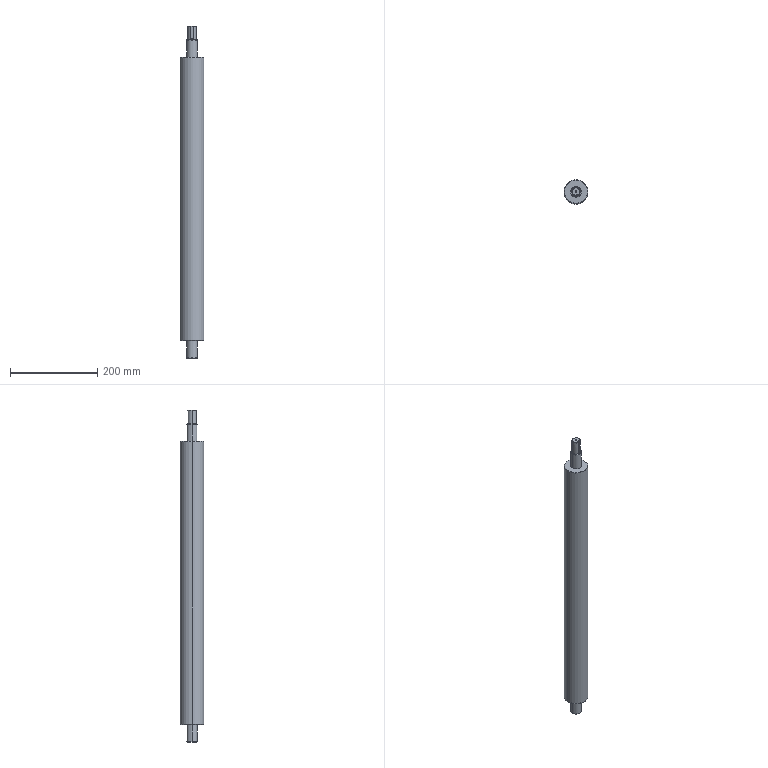Part | SolidWorks | features ICE 3, Chamfer 2, Extrusion 1, HoleWzd 1, MirrorPattern 1 | 1 solid | 32 faces | box 55 x 55 x 762 mm | volume 1592560 mm3 | cone 13 | cylinder 11 | plane 8 | commonest cylinder face diameters 25 x4 4.2 x2 20 x2 55 x2 6 x1
STEP:
#1=CARTESIAN_POINT('',(-2.1,0.,384.6));
#2=VERTEX_POINT('',#1);
#3=CARTESIAN_POINT('',(2.1,0.,384.6));
#4=VERTEX_POINT('',#3);
#5=CARTESIAN_POINT('',(0.,0.,384.6));
#6=DIRECTION('',(0.,0.,1.));
#7=DIRECTION('',(1.,0.,0.));
#8=AXIS2_PLACEMENT_3D('',#5,#6,#7);
#9=CIRCLE('',#8,2.1);
#10=EDGE_CURVE('',#2,#4,#9,.T.);
#11=ORIENTED_EDGE('',*,*,#10,.F.);
#12=CARTESIAN_POINT('',(-2.1,0.,397.));
#13=VERTEX_POINT('',#12);
#14=CARTESIAN_POINT('',(-2.1,0.,397.));
#15=DIRECTION('',(0.,0.,1.));
#16=VECTOR('',#15,1000.);
#17=LINE('',#14,#16);
#18=EDGE_CURVE('',#2,#13,#17,.T.);
#19=ORIENTED_EDGE('',*,*,#18,.T.);
#20=CARTESIAN_POINT('',(2.1,0.,397.));
#21=VERTEX_POINT('',#20);
#22=CARTESIAN_POINT('',(0.,0.,397.));
#23=DIRECTION('',(0.,0.,1.));
#24=DIRECTION('',(1.,0.,0.));
#25=AXIS2_PLACEMENT_3D('',#22,#23,#24);
#26=CIRCLE('',#25,2.1);
#27=EDGE_CURVE('',#13,#21,#26,.T.);
#28=ORIENTED_EDGE('',*,*,#27,.T.);
#29=CARTESIAN_POINT('',(2.1,0.,397.));
#30=DIRECTION('',(0.,0.,1.));
#31=VECTOR('',#30,1000.);
#32=LINE('',#29,#31);
#33=EDGE_CURVE('',#4,#21,#32,.T.);
#34=ORIENTED_EDGE('',*,*,#33,.F.);
#35=EDGE_LOOP('',(#11,#19,#28,#34));
#36=FACE_OUTER_BOUND('',#35,.T.);
#37=CARTESIAN_POINT('',(0.,0.,397.));
#38=DIRECTION('',(0.,0.,1.));
#39=DIRECTION('',(1.,0.,0.));
#40=AXIS2_PLACEMENT_3D('',#37,#38,#39);
#41=CYLINDRICAL_SURFACE('',#40,2.1);
#42=ADVANCED_FACE('',(#36),#41,.F.);
#43=CARTESIAN_POINT('',(0.,0.,383.338));
#44=VERTEX_POINT('',#43);
#45=CARTESIAN_POINT('',(2.1,0.,384.6));
#46=DIRECTION('',(0.8572,0.,0.515));
#47=VECTOR('',#46,1000.);
#48=LINE('',#45,#47);
#49=EDGE_CURVE('',#44,#4,#48,.T.);
#50=ORIENTED_EDGE('',*,*,#49,.F.);
#51=CARTESIAN_POINT('',(-2.1,0.,384.6));
#52=DIRECTION('',(-0.8572,0.,0.515));
#53=VECTOR('',#52,1000.);
#54=LINE('',#51,#53);
#55=EDGE_CURVE('',#44,#2,#54,.T.);
#56=ORIENTED_EDGE('',*,*,#55,.T.);
#57=ORIENTED_EDGE('',*,*,#10,.T.);
#58=EDGE_LOOP('',(#50,#56,#57));
#59=FACE_OUTER_BOUND('',#58,.T.);
#60=CARTESIAN_POINT('',(0.,0.,384.6));
#61=DIRECTION('',(0.,0.,1.));
#62=DIRECTION('',(1.,0.,0.));
#63=AXIS2_PLACEMENT_3D('',#60,#61,#62);
#64=CONICAL_SURFACE('',#63,2.1,1.03);
#65=ADVANCED_FACE('',(#59),#64,.F.);
#66=CARTESIAN_POINT('',(9.,0.,397.));
#67=VERTEX_POINT('',#66);
#68=CARTESIAN_POINT('',(-9.,0.,397.));
#69=VERTEX_POINT('',#68);
#70=CARTESIAN_POINT('',(0.,0.,397.));
#71=DIRECTION('',(0.,0.,1.));
#72=DIRECTION('',(1.,0.,0.));
#73=AXIS2_PLACEMENT_3D('',#70,#71,#72);
#74=CIRCLE('',#73,9.);
#75=EDGE_CURVE('',#67,#69,#74,.T.);
#76=ORIENTED_EDGE('',*,*,#75,.F.);
#77=CARTESIAN_POINT('',(10.,0.,396.));
#78=VERTEX_POINT('',#77);
#79=CARTESIAN_POINT('',(9.,0.,397.));
#80=DIRECTION('',(0.7071,0.,-0.7071));
#81=VECTOR('',#80,1000.);
#82=LINE('',#79,#81);
#83=EDGE_CURVE('',#67,#78,#82,.T.);
#84=ORIENTED_EDGE('',*,*,#83,.T.);
#85=CARTESIAN_POINT('',(-10.,0.,396.));
#86=VERTEX_POINT('',#85);
#87=CARTESIAN_POINT('',(0.,0.,396.));
#88=DIRECTION('',(0.,0.,-1.));
#89=DIRECTION('',(1.,0.,0.));
#90=AXIS2_PLACEMENT_3D('',#87,#88,#89);
#91=CIRCLE('',#90,10.);
#92=EDGE_CURVE('',#86,#78,#91,.T.);
#93=ORIENTED_EDGE('',*,*,#92,.F.);
#94=CARTESIAN_POINT('',(-9.,0.,397.));
#95=DIRECTION('',(-0.7071,0.,-0.7071));
#96=VECTOR('',#95,1000.);
#97=LINE('',#94,#96);
#98=EDGE_CURVE('',#69,#86,#97,.T.);
#99=ORIENTED_EDGE('',*,*,#98,.F.);
#100=EDGE_LOOP('',(#76,#84,#93,#99));
#101=FACE_OUTER_BOUND('',#100,.T.);
#102=CARTESIAN_POINT('',(0.,0.,397.));
#103=DIRECTION('',(0.,0.,-1.));
#104=DIRECTION('',(-1.,0.,0.));
#105=AXIS2_PLACEMENT_3D('',#102,#103,#104);
#106=CONICAL_SURFACE('',#105,9.,0.7854);
#107=ADVANCED_FACE('',(#101),#106,.T.);
#108=CARTESIAN_POINT('',(-3.,-8.485,397.));
#109=VERTEX_POINT('',#108);
#110=CARTESIAN_POINT('',(0.,0.,397.));
#111=DIRECTION('',(0.,0.,1.));
#112=DIRECTION('',(1.,0.,0.));
#113=AXIS2_PLACEMENT_3D('',#110,#111,#112);
#114=CIRCLE('',#113,9.);
#115=EDGE_CURVE('',#69,#109,#114,.T.);
#116=ORIENTED_EDGE('',*,*,#115,.F.);
#117=ORIENTED_EDGE('',*,*,#98,.T.);
#118=CARTESIAN_POINT('',(-3.,-9.539,396.));
#119=VERTEX_POINT('',#118);
#120=CARTESIAN_POINT('',(0.,0.,396.));
#121=DIRECTION('',(0.,0.,-1.));
#122=DIRECTION('',(1.,0.,0.));
#123=AXIS2_PLACEMENT_3D('',#120,#121,#122);
#124=CIRCLE('',#123,10.);
#125=EDGE_CURVE('',#119,#86,#124,.T.);
#126=ORIENTED_EDGE('',*,*,#125,.F.);
#127=CARTESIAN_POINT('',(-3.,-8.485,397.));
#128=CARTESIAN_POINT('',(-3.,-8.838,396.668));
#129=CARTESIAN_POINT('',(-3.,-9.189,396.334));
#130=CARTESIAN_POINT('',(-3.,-9.539,396.));
#131=B_SPLINE_CURVE_WITH_KNOTS('',3,(#127,#128,#129,#130),.UNSPECIFIED.,.F.,.F.,(4,4),(0.005441,0.006894),.UNSPECIFIED.);
#132=EDGE_CURVE('',#109,#119,#131,.T.);
#133=ORIENTED_EDGE('',*,*,#132,.F.);
#134=EDGE_LOOP('',(#116,#117,#126,#133));
#135=FACE_OUTER_BOUND('',#134,.T.);
#136=CARTESIAN_POINT('',(0.,0.,397.));
#137=DIRECTION('',(0.,0.,-1.));
#138=DIRECTION('',(-1.,0.,0.));
#139=AXIS2_PLACEMENT_3D('',#136,#137,#138);
#140=CONICAL_SURFACE('',#139,9.,0.7854);
#141=ADVANCED_FACE('',(#135),#140,.T.);
#142=ORIENTED_EDGE('',*,*,#92,.T.);
#143=CARTESIAN_POINT('',(10.,0.,365.));
#144=VERTEX_POINT('',#143);
#145=CARTESIAN_POINT('',(10.,0.,397.));
#146=DIRECTION('',(0.,0.,-1.));
#147=VECTOR('',#146,1000.);
#148=LINE('',#145,#147);
#149=EDGE_CURVE('',#78,#144,#148,.T.);
#150=ORIENTED_EDGE('',*,*,#149,.T.);
#151=CARTESIAN_POINT('',(-10.,0.,365.));
#152=VERTEX_POINT('',#151);
#153=CARTESIAN_POINT('',(0.,0.,365.));
#154=DIRECTION('',(0.,0.,1.));
#155=DIRECTION('',(1.,0.,0.));
#156=AXIS2_PLACEMENT_3D('',#153,#154,#155);
#157=CIRCLE('',#156,10.);
#158=EDGE_CURVE('',#144,#152,#157,.T.);
#159=ORIENTED_EDGE('',*,*,#158,.T.);
#160=CARTESIAN_POINT('',(-10.,0.,397.));
#161=DIRECTION('',(0.,0.,-1.));
#162=VECTOR('',#161,1000.);
#163=LINE('',#160,#162);
#164=EDGE_CURVE('',#86,#152,#163,.T.);
#165=ORIENTED_EDGE('',*,*,#164,.F.);
#166=EDGE_LOOP('',(#142,#150,#159,#165));
#167=FACE_OUTER_BOUND('',#166,.T.);
#168=CARTESIAN_POINT('',(0.,0.,397.));
#169=DIRECTION('',(0.,0.,-1.));
#170=DIRECTION('',(-1.,0.,0.));
#171=AXIS2_PLACEMENT_3D('',#168,#169,#170);
#172=CYLINDRICAL_SURFACE('',#171,10.);
#173=ADVANCED_FACE('',(#167),#172,.T.);
#174=CARTESIAN_POINT('',(26.5,0.,325.));
#175=VERTEX_POINT('',#174);
#176=CARTESIAN_POINT('',(-26.5,0.,325.));
#177=VERTEX_POINT('',#176);
#178=CARTESIAN_POINT('',(0.,0.,325.));
#179=DIRECTION('',(0.,0.,1.));
#180=DIRECTION('',(1.,0.,0.));
#181=AXIS2_PLACEMENT_3D('',#178,#179,#180);
#182=CIRCLE('',#181,26.5);
#183=EDGE_CURVE('',#175,#177,#182,.T.);
#184=ORIENTED_EDGE('',*,*,#183,.F.);
#185=CARTESIAN_POINT('',(27.5,0.,324.));
#186=VERTEX_POINT('',#185);
#187=CARTESIAN_POINT('',(26.5,0.,325.));
#188=DIRECTION('',(0.7071,0.,-0.7071));
#189=VECTOR('',#188,1000.);
#190=LINE('',#187,#189);
#191=EDGE_CURVE('',#175,#186,#190,.T.);
#192=ORIENTED_EDGE('',*,*,#191,.T.);
#193=CARTESIAN_POINT('',(-27.5,0.,324.));
#194=VERTEX_POINT('',#193);
#195=CARTESIAN_POINT('',(0.,0.,324.));
#196=DIRECTION('',(0.,0.,-1.));
#197=DIRECTION('',(1.,0.,0.));
#198=AXIS2_PLACEMENT_3D('',#195,#196,#197);
#199=CIRCLE('',#198,27.5);
#200=EDGE_CURVE('',#194,#186,#199,.T.);
#201=ORIENTED_EDGE('',*,*,#200,.F.);
#202=CARTESIAN_POINT('',(-26.5,0.,325.));
#203=DIRECTION('',(-0.7071,0.,-0.7071));
#204=VECTOR('',#203,1000.);
#205=LINE('',#202,#204);
#206=EDGE_CURVE('',#177,#194,#205,.T.);
#207=ORIENTED_EDGE('',*,*,#206,.F.);
#208=EDGE_LOOP('',(#184,#192,#201,#207));
#209=FACE_OUTER_BOUND('',#208,.T.);
#210=CARTESIAN_POINT('',(0.,0.,325.));
#211=DIRECTION('',(0.,0.,-1.));
#212=DIRECTION('',(-1.,0.,0.));
#213=AXIS2_PLACEMENT_3D('',#210,#211,#212);
#214=CONICAL_SURFACE('',#213,26.5,0.7854);
#215=ADVANCED_FACE('',(#209),#214,.T.);
#216=CARTESIAN_POINT('',(11.5,0.,365.));
#217=VERTEX_POINT('',#216);
#218=CARTESIAN_POINT('',(-11.5,0.,365.));
#219=VERTEX_POINT('',#218);
#220=CARTESIAN_POINT('',(0.,0.,365.));
#221=DIRECTION('',(0.,0.,1.));
#222=DIRECTION('',(1.,0.,0.));
#223=AXIS2_PLACEMENT_3D('',#220,#221,#222);
#224=CIRCLE('',#223,11.5);
#225=EDGE_CURVE('',#217,#219,#224,.T.);
#226=ORIENTED_EDGE('',*,*,#225,.F.);
#227=CARTESIAN_POINT('',(12.5,0.,364.));
#228=VERTEX_POINT('',#227);
#229=CARTESIAN_POINT('',(11.5,0.,365.));
#230=DIRECTION('',(0.7071,0.,-0.7071));
#231=VECTOR('',#230,1000.);
#232=LINE('',#229,#231);
#233=EDGE_CURVE('',#217,#228,#232,.T.);
#234=ORIENTED_EDGE('',*,*,#233,.T.);
#235=CARTESIAN_POINT('',(-12.5,0.,364.));
#236=VERTEX_POINT('',#235);
#237=CARTESIAN_POINT('',(0.,0.,364.));
#238=DIRECTION('',(0.,0.,-1.));
#239=DIRECTION('',(1.,0.,0.));
#240=AXIS2_PLACEMENT_3D('',#237,#238,#239);
#241=CIRCLE('',#240,12.5);
#242=EDGE_CURVE('',#236,#228,#241,.T.);
#243=ORIENTED_EDGE('',*,*,#242,.F.);
#244=CARTESIAN_POINT('',(-11.5,0.,365.));
#245=DIRECTION('',(-0.7071,0.,-0.7071));
#246=VECTOR('',#245,1000.);
#247=LINE('',#244,#246);
#248=EDGE_CURVE('',#219,#236,#247,.T.);
#249=ORIENTED_EDGE('',*,*,#248,.F.);
#250=EDGE_LOOP('',(#226,#234,#243,#249));
#251=FACE_OUTER_BOUND('',#250,.T.);
#252=CARTESIAN_POINT('',(0.,0.,365.));
#253=DIRECTION('',(0.,0.,-1.));
#254=DIRECTION('',(-1.,0.,0.));
#255=AXIS2_PLACEMENT_3D('',#252,#253,#254);
#256=CONICAL_SURFACE('',#255,11.5,0.7854);
#257=ADVANCED_FACE('',(#251),#256,.T.);
#258=CARTESIAN_POINT('',(-26.5,0.,-325.));
#259=VERTEX_POINT('',#258);
#260=CARTESIAN_POINT('',(26.5,0.,-325.));
#261=VERTEX_POINT('',#260);
#262=CARTESIAN_POINT('',(0.,0.,-325.));
#263=DIRECTION('',(0.,0.,-1.));
#264=DIRECTION('',(1.,0.,0.));
#265=AXIS2_PLACEMENT_3D('',#262,#263,#264);
#266=CIRCLE('',#265,26.5);
#267=EDGE_CURVE('',#259,#261,#266,.T.);
#268=ORIENTED_EDGE('',*,*,#267,.F.);
#269=CARTESIAN_POINT('',(-27.5,0.,-324.));
#270=VERTEX_POINT('',#269);
#271=CARTESIAN_POINT('',(-27.5,0.,-324.));
#272=DIRECTION('',(-0.7071,0.,0.7071));
#273=VECTOR('',#272,1000.);
#274=LINE('',#271,#273);
#275=EDGE_CURVE('',#259,#270,#274,.T.);
#276=ORIENTED_EDGE('',*,*,#275,.T.);
#277=CARTESIAN_POINT('',(27.5,0.,-324.));
#278=VERTEX_POINT('',#277);
#279=CARTESIAN_POINT('',(0.,0.,-324.));
#280=DIRECTION('',(0.,0.,1.));
#281=DIRECTION('',(1.,0.,0.));
#282=AXIS2_PLACEMENT_3D('',#279,#280,#281);
#283=CIRCLE('',#282,27.5);
#284=EDGE_CURVE('',#278,#270,#283,.T.);
#285=ORIENTED_EDGE('',*,*,#284,.F.);
#286=CARTESIAN_POINT('',(27.5,0.,-324.));
#287=DIRECTION('',(0.7071,0.,0.7071));
#288=VECTOR('',#287,1000.);
#289=LINE('',#286,#288);
#290=EDGE_CURVE('',#261,#278,#289,.T.);
#291=ORIENTED_EDGE('',*,*,#290,.F.);
#292=EDGE_LOOP('',(#268,#276,#285,#291));
#293=FACE_OUTER_BOUND('',#292,.T.);
#294=CARTESIAN_POINT('',(0.,0.,-324.));
#295=DIRECTION('',(0.,0.,1.));
#296=DIRECTION('',(1.,0.,0.));
#297=AXIS2_PLACEMENT_3D('',#294,#295,#296);
#298=CONICAL_SURFACE('',#297,27.5,0.7854);
#299=ADVANCED_FACE('',(#293),#298,.T.);
#300=CARTESIAN_POINT('',(-11.5,0.,-365.));
#301=VERTEX_POINT('',#300);
#302=CARTESIAN_POINT('',(11.5,0.,-365.));
#303=VERTEX_POINT('',#302);
#304=CARTESIAN_POINT('',(0.,0.,-365.));
#305=DIRECTION('',(0.,0.,-1.));
#306=DIRECTION('',(-1.,0.,0.));
#307=AXIS2_PLACEMENT_3D('',#304,#305,#306);
#308=CIRCLE('',#307,11.5);
#309=EDGE_CURVE('',#301,#303,#308,.T.);
#310=ORIENTED_EDGE('',*,*,#309,.F.);
#311=CARTESIAN_POINT('',(-12.5,0.,-364.));
#312=VERTEX_POINT('',#311);
#313=CARTESIAN_POINT('',(-12.5,0.,-364.));
#314=DIRECTION('',(-0.7071,0.,0.7071));
#315=VECTOR('',#314,1000.);
#316=LINE('',#313,#315);
#317=EDGE_CURVE('',#301,#312,#316,.T.);
#318=ORIENTED_EDGE('',*,*,#317,.T.);
#319=CARTESIAN_POINT('',(12.5,0.,-364.));
#320=VERTEX_POINT('',#319);
#321=CARTESIAN_POINT('',(0.,0.,-364.));
#322=DIRECTION('',(0.,0.,1.));
#323=DIRECTION('',(-1.,0.,0.));
#324=AXIS2_PLACEMENT_3D('',#321,#322,#323);
#325=CIRCLE('',#324,12.5);
#326=EDGE_CURVE('',#320,#312,#325,.T.);
#327=ORIENTED_EDGE('',*,*,#326,.F.);
#328=CARTESIAN_POINT('',(12.5,0.,-364.));
#329=DIRECTION('',(0.7071,0.,0.7071));
#330=VECTOR('',#329,1000.);
#331=LINE('',#328,#330);
#332=EDGE_CURVE('',#303,#320,#331,.T.);
#333=ORIENTED_EDGE('',*,*,#332,.F.);
#334=EDGE_LOOP('',(#310,#318,#327,#333));
#335=FACE_OUTER_BOUND('',#334,.T.);
#336=CARTESIAN_POINT('',(0.,0.,-364.));
#337=DIRECTION('',(0.,0.,1.));
#338=DIRECTION('',(1.,0.,0.));
#339=AXIS2_PLACEMENT_3D('',#336,#337,#338);
#340=CONICAL_SURFACE('',#339,12.5,0.7854);
#341=ADVANCED_FACE('',(#335),#340,.T.);
#342=ORIENTED_EDGE('',*,*,#326,.T.);
#343=CARTESIAN_POINT('',(-12.5,0.,-325.));
#344=VERTEX_POINT('',#343);
#345=CARTESIAN_POINT('',(-12.5,0.,-365.));
#346=DIRECTION('',(0.,0.,1.));
#347=VECTOR('',#346,1000.);
#348=LINE('',#345,#347);
#349=EDGE_CURVE('',#312,#344,#348,.T.);
#350=ORIENTED_EDGE('',*,*,#349,.T.);
#351=CARTESIAN_POINT('',(12.5,0.,-325.));
#352=VERTEX_POINT('',#351);
#353=CARTESIAN_POINT('',(0.,0.,-325.));
#354=DIRECTION('',(0.,0.,1.));
#355=DIRECTION('',(1.,0.,0.));
#356=AXIS2_PLACEMENT_3D('',#353,#354,#355);
#357=CIRCLE('',#356,12.5);
#358=EDGE_CURVE('',#352,#344,#357,.T.);
#359=ORIENTED_EDGE('',*,*,#358,.F.);
#360=CARTESIAN_POINT('',(12.5,0.,-365.));
#361=DIRECTION('',(0.,0.,1.));
#362=VECTOR('',#361,1000.);
#363=LINE('',#360,#362);
#364=EDGE_CURVE('',#320,#352,#363,.T.);
#365=ORIENTED_EDGE('',*,*,#364,.F.);
#366=EDGE_LOOP('',(#342,#350,#359,#365));
#367=FACE_OUTER_BOUND('',#366,.T.);
#368=CARTESIAN_POINT('',(0.,0.,-365.));
#369=DIRECTION('',(0.,0.,1.));
#370=DIRECTION('',(1.,0.,0.));
#371=AXIS2_PLACEMENT_3D('',#368,#369,#370);
#372=CYLINDRICAL_SURFACE('',#371,12.5);
#373=ADVANCED_FACE('',(#367),#372,.T.);
#374=ORIENTED_EDGE('',*,*,#242,.T.);
#375=CARTESIAN_POINT('',(12.5,0.,325.));
#376=VERTEX_POINT('',#375);
#377=CARTESIAN_POINT('',(12.5,0.,365.));
#378=DIRECTION('',(0.,0.,-1.));
#379=VECTOR('',#378,1000.);
#380=LINE('',#377,#379);
#381=EDGE_CURVE('',#228,#376,#380,.T.);
#382=ORIENTED_EDGE('',*,*,#381,.T.);
#383=CARTESIAN_POINT('',(-12.5,0.,325.));
#384=VERTEX_POINT('',#383);
#385=CARTESIAN_POINT('',(0.,0.,325.));
#386=DIRECTION('',(0.,0.,1.));
#387=DIRECTION('',(1.,0.,0.));
#388=AXIS2_PLACEMENT_3D('',#385,#386,#387);
#389=CIRCLE('',#388,12.5);
#390=EDGE_CURVE('',#376,#384,#389,.T.);
#391=ORIENTED_EDGE('',*,*,#390,.T.);
#392=CARTESIAN_POINT('',(-12.5,0.,365.));
#393=DIRECTION('',(0.,0.,-1.));
#394=VECTOR('',#393,1000.);
#395=LINE('',#392,#394);
#396=EDGE_CURVE('',#236,#384,#395,.T.);
#397=ORIENTED_EDGE('',*,*,#396,.F.);
#398=EDGE_LOOP('',(#374,#382,#391,#397));
#399=FACE_OUTER_BOUND('',#398,.T.);
#400=CARTESIAN_POINT('',(0.,0.,365.));
#401=DIRECTION('',(0.,0.,-1.));
#402=DIRECTION('',(-1.,0.,0.));
#403=AXIS2_PLACEMENT_3D('',#400,#401,#402);
#404=CYLINDRICAL_SURFACE('',#403,12.5);
#405=ADVANCED_FACE('',(#399),#404,.T.);
#406=ORIENTED_EDGE('',*,*,#200,.T.);
#407=CARTESIAN_POINT('',(27.5,0.,325.));
#408=DIRECTION('',(0.,0.,-1.));
#409=VECTOR('',#408,1000.);
#410=LINE('',#407,#409);
#411=EDGE_CURVE('',#186,#278,#410,.T.);
#412=ORIENTED_EDGE('',*,*,#411,.T.);
#413=ORIENTED_EDGE('',*,*,#284,.T.);
#414=CARTESIAN_POINT('',(-27.5,0.,325.));
#415=DIRECTION('',(0.,0.,-1.));
#416=VECTOR('',#415,1000.);
#417=LINE('',#414,#416);
#418=EDGE_CURVE('',#194,#270,#417,.T.);
#419=ORIENTED_EDGE('',*,*,#418,.F.);
#420=EDGE_LOOP('',(#406,#412,#413,#419));
#421=FACE_OUTER_BOUND('',#420,.T.);
#422=CARTESIAN_POINT('',(0.,0.,325.));
#423=DIRECTION('',(0.,0.,-1.));
#424=DIRECTION('',(-1.,0.,0.));
#425=AXIS2_PLACEMENT_3D('',#422,#423,#424);
#426=CYLINDRICAL_SURFACE('',#425,27.5);
#427=ADVANCED_FACE('',(#421),#426,.T.);
#428=ORIENTED_EDGE('',*,*,#411,.F.);
#429=CARTESIAN_POINT('',(0.,0.,324.));
#430=DIRECTION('',(0.,0.,-1.));
#431=DIRECTION('',(1.,0.,0.));
#432=AXIS2_PLACEMENT_3D('',#429,#430,#431);
#433=CIRCLE('',#432,27.5);
#434=EDGE_CURVE('',#186,#194,#433,.T.);
#435=ORIENTED_EDGE('',*,*,#434,.T.);
#436=ORIENTED_EDGE('',*,*,#418,.T.);
#437=CARTESIAN_POINT('',(0.,0.,-324.));
#438=DIRECTION('',(0.,0.,1.));
#439=DIRECTION('',(1.,0.,0.));
#440=AXIS2_PLACEMENT_3D('',#437,#438,#439);
#441=CIRCLE('',#440,27.5);
#442=EDGE_CURVE('',#270,#278,#441,.T.);
#443=ORIENTED_EDGE('',*,*,#442,.T.);
#444=EDGE_LOOP('',(#428,#435,#436,#443));
#445=FACE_OUTER_BOUND('',#444,.T.);
#446=CARTESIAN_POINT('',(0.,0.,325.));
#447=DIRECTION('',(0.,0.,-1.));
#448=DIRECTION('',(-1.,0.,0.));
#449=AXIS2_PLACEMENT_3D('',#446,#447,#448);
#450=CYLINDRICAL_SURFACE('',#449,27.5);
#451=ADVANCED_FACE('',(#445),#450,.T.);
#452=CARTESIAN_POINT('',(0.,0.,325.));
#453=DIRECTION('',(0.,0.,1.));
#454=DIRECTION('',(1.,0.,0.));
#455=AXIS2_PLACEMENT_3D('',#452,#453,#454);
#456=CIRCLE('',#455,26.5);
#457=EDGE_CURVE('',#177,#175,#456,.T.);
#458=ORIENTED_EDGE('',*,*,#457,.T.);
#459=ORIENTED_EDGE('',*,*,#183,.T.);
#460=EDGE_LOOP('',(#458,#459));
#461=FACE_OUTER_BOUND('',#460,.T.);
#462=CARTESIAN_POINT('',(0.,0.,325.));
#463=DIRECTION('',(0.,0.,1.));
#464=DIRECTION('',(1.,0.,0.));
#465=AXIS2_PLACEMENT_3D('',#462,#463,#464);
#466=CIRCLE('',#465,12.5);
#467=EDGE_CURVE('',#384,#376,#466,.T.);
#468=ORIENTED_EDGE('',*,*,#467,.F.);
#469=ORIENTED_EDGE('',*,*,#390,.F.);
#470=EDGE_LOOP('',(#468,#469));
#471=FACE_BOUND('',#470,.T.);
#472=CARTESIAN_POINT('',(0.,0.,325.));
#473=DIRECTION('',(0.,0.,1.));
#474=DIRECTION('',(1.,0.,0.));
#475=AXIS2_PLACEMENT_3D('',#472,#473,#474);
#476=PLANE('',#475);
#477=ADVANCED_FACE('',(#461,#471),#476,.T.);
#478=CARTESIAN_POINT('',(0.,0.,-325.));
#479=DIRECTION('',(0.,0.,-1.));
#480=DIRECTION('',(1.,0.,0.));
#481=AXIS2_PLACEMENT_3D('',#478,#479,#480);
#482=CIRCLE('',#481,26.5);
#483=EDGE_CURVE('',#261,#259,#482,.T.);
#484=ORIENTED_EDGE('',*,*,#483,.T.);
#485=ORIENTED_EDGE('',*,*,#267,.T.);
#486=EDGE_LOOP('',(#484,#485));
#487=FACE_OUTER_BOUND('',#486,.T.);
#488=ORIENTED_EDGE('',*,*,#358,.T.);
#489=CARTESIAN_POINT('',(0.,0.,-325.));
#490=DIRECTION('',(0.,0.,1.));
#491=DIRECTION('',(1.,0.,0.));
#492=AXIS2_PLACEMENT_3D('',#489,#490,#491);
#493=CIRCLE('',#492,12.5);
#494=EDGE_CURVE('',#344,#352,#493,.T.);
#495=ORIENTED_EDGE('',*,*,#494,.T.);
#496=EDGE_LOOP('',(#488,#495));
#497=FACE_BOUND('',#496,.T.);
#498=CARTESIAN_POINT('',(0.,0.,-325.));
#499=DIRECTION('',(0.,0.,1.));
#500=DIRECTION('',(1.,0.,0.));
#501=AXIS2_PLACEMENT_3D('',#498,#499,#500);
#502=PLANE('',#501);
#503=ADVANCED_FACE('',(#487,#497),#502,.F.);
#504=ORIENTED_EDGE('',*,*,#381,.F.);
#505=CARTESIAN_POINT('',(0.,0.,364.));
#506=DIRECTION('',(0.,0.,-1.));
#507=DIRECTION('',(1.,0.,0.));
#508=AXIS2_PLACEMENT_3D('',#505,#506,#507);
#509=CIRCLE('',#508,12.5);
#510=EDGE_CURVE('',#228,#236,#509,.T.);
#511=ORIENTED_EDGE('',*,*,#510,.T.);
#512=ORIENTED_EDGE('',*,*,#396,.T.);
#513=ORIENTED_EDGE('',*,*,#467,.T.);
#514=EDGE_LOOP('',(#504,#511,#512,#513));
#515=FACE_OUTER_BOUND('',#514,.T.);
#516=CARTESIAN_POINT('',(0.,0.,365.));
#517=DIRECTION('',(0.,0.,-1.));
#518=DIRECTION('',(-1.,0.,0.));
#519=AXIS2_PLACEMENT_3D('',#516,#517,#518);
#520=CYLINDRICAL_SURFACE('',#519,12.5);
#521=ADVANCED_FACE('',(#515),#520,.T.);
#522=CARTESIAN_POINT('',(0.,0.,365.));
#523=DIRECTION('',(0.,0.,1.));
#524=DIRECTION('',(1.,0.,0.));
#525=AXIS2_PLACEMENT_3D('',#522,#523,#524);
#526=CIRCLE('',#525,10.);
#527=EDGE_CURVE('',#152,#144,#526,.T.);
#528=ORIENTED_EDGE('',*,*,#527,.F.);
#529=ORIENTED_EDGE('',*,*,#158,.F.);
#530=EDGE_LOOP('',(#528,#529));
#531=FACE_BOUND('',#530,.T.);
#532=CARTESIAN_POINT('',(0.,0.,365.));
#533=DIRECTION('',(0.,0.,1.));
#534=DIRECTION('',(1.,0.,0.));
#535=AXIS2_PLACEMENT_3D('',#532,#533,#534);
#536=CIRCLE('',#535,11.5);
#537=EDGE_CURVE('',#219,#217,#536,.T.);
#538=ORIENTED_EDGE('',*,*,#537,.T.);
#539=ORIENTED_EDGE('',*,*,#225,.T.);
#540=EDGE_LOOP('',(#538,#539));
#541=FACE_OUTER_BOUND('',#540,.T.);
#542=CARTESIAN_POINT('',(0.,0.,365.));
#543=DIRECTION('',(0.,0.,1.));
#544=DIRECTION('',(1.,0.,0.));
#545=AXIS2_PLACEMENT_3D('',#542,#543,#544);
#546=PLANE('',#545);
#547=ADVANCED_FACE('',(#531,#541),#546,.T.);
#548=ORIENTED_EDGE('',*,*,#349,.F.);
#549=CARTESIAN_POINT('',(0.,0.,-364.));
#550=DIRECTION('',(0.,0.,1.));
#551=DIRECTION('',(-1.,0.,0.));
#552=AXIS2_PLACEMENT_3D('',#549,#550,#551);
#553=CIRCLE('',#552,12.5);
#554=EDGE_CURVE('',#312,#320,#553,.T.);
#555=ORIENTED_EDGE('',*,*,#554,.T.);
#556=ORIENTED_EDGE('',*,*,#364,.T.);
#557=ORIENTED_EDGE('',*,*,#494,.F.);
#558=EDGE_LOOP('',(#548,#555,#556,#557));
#559=FACE_OUTER_BOUND('',#558,.T.);
#560=CARTESIAN_POINT('',(0.,0.,-365.));
#561=DIRECTION('',(0.,0.,1.));
#562=DIRECTION('',(1.,0.,0.));
#563=AXIS2_PLACEMENT_3D('',#560,#561,#562);
#564=CYLINDRICAL_SURFACE('',#563,12.5);
#565=ADVANCED_FACE('',(#559),#564,.T.);
#566=CARTESIAN_POINT('',(0.,0.,-365.));
#567=DIRECTION('',(0.,0.,-1.));
#568=DIRECTION('',(-1.,0.,0.));
#569=AXIS2_PLACEMENT_3D('',#566,#567,#568);
#570=CIRCLE('',#569,11.5);
#571=EDGE_CURVE('',#303,#301,#570,.T.);
#572=ORIENTED_EDGE('',*,*,#571,.T.);
#573=ORIENTED_EDGE('',*,*,#309,.T.);
#574=EDGE_LOOP('',(#572,#573));
#575=FACE_OUTER_BOUND('',#574,.T.);
#576=CARTESIAN_POINT('',(0.,0.,-365.));
#577=DIRECTION('',(0.,0.,-1.));
#578=DIRECTION('',(1.,0.,0.));
#579=AXIS2_PLACEMENT_3D('',#576,#577,#578);
#580=PLANE('',#579);
#581=ADVANCED_FACE('',(#575),#580,.T.);
#582=ORIENTED_EDGE('',*,*,#317,.F.);
#583=ORIENTED_EDGE('',*,*,#571,.F.);
#584=ORIENTED_EDGE('',*,*,#332,.T.);
#585=ORIENTED_EDGE('',*,*,#554,.F.);
#586=EDGE_LOOP('',(#582,#583,#584,#585));
#587=FACE_OUTER_BOUND('',#586,.T.);
#588=CARTESIAN_POINT('',(0.,0.,-364.));
#589=DIRECTION('',(0.,0.,1.));
#590=DIRECTION('',(1.,0.,0.));
#591=AXIS2_PLACEMENT_3D('',#588,#589,#590);
#592=CONICAL_SURFACE('',#591,12.5,0.7854);
#593=ADVANCED_FACE('',(#587),#592,.T.);
#594=ORIENTED_EDGE('',*,*,#275,.F.);
#595=ORIENTED_EDGE('',*,*,#483,.F.);
#596=ORIENTED_EDGE('',*,*,#290,.T.);
#597=ORIENTED_EDGE('',*,*,#442,.F.);
#598=EDGE_LOOP('',(#594,#595,#596,#597));
#599=FACE_OUTER_BOUND('',#598,.T.);
#600=CARTESIAN_POINT('',(0.,0.,-324.));
#601=DIRECTION('',(0.,0.,1.));
#602=DIRECTION('',(1.,0.,0.));
#603=AXIS2_PLACEMENT_3D('',#600,#601,#602);
#604=CONICAL_SURFACE('',#603,27.5,0.7854);
#605=ADVANCED_FACE('',(#599),#604,.T.);
#606=ORIENTED_EDGE('',*,*,#233,.F.);
#607=ORIENTED_EDGE('',*,*,#537,.F.);
#608=ORIENTED_EDGE('',*,*,#248,.T.);
#609=ORIENTED_EDGE('',*,*,#510,.F.);
#610=EDGE_LOOP('',(#606,#607,#608,#609));
#611=FACE_OUTER_BOUND('',#610,.T.);
#612=CARTESIAN_POINT('',(0.,0.,365.));
#613=DIRECTION('',(0.,0.,-1.));
#614=DIRECTION('',(-1.,0.,0.));
#615=AXIS2_PLACEMENT_3D('',#612,#613,#614);
#616=CONICAL_SURFACE('',#615,11.5,0.7854);
#617=ADVANCED_FACE('',(#611),#616,.T.);
#618=ORIENTED_EDGE('',*,*,#191,.F.);
#619=ORIENTED_EDGE('',*,*,#457,.F.);
#620=ORIENTED_EDGE('',*,*,#206,.T.);
#621=ORIENTED_EDGE('',*,*,#434,.F.);
#622=EDGE_LOOP('',(#618,#619,#620,#621));
#623=FACE_OUTER_BOUND('',#622,.T.);
#624=CARTESIAN_POINT('',(0.,0.,325.));
#625=DIRECTION('',(0.,0.,-1.));
#626=DIRECTION('',(-1.,0.,0.));
#627=AXIS2_PLACEMENT_3D('',#624,#625,#626);
#628=CONICAL_SURFACE('',#627,26.5,0.7854);
#629=ADVANCED_FACE('',(#623),#628,.T.);
#630=ORIENTED_EDGE('',*,*,#149,.F.);
#631=CARTESIAN_POINT('',(3.,-9.539,396.));
#632=VERTEX_POINT('',#631);
#633=CARTESIAN_POINT('',(0.,0.,396.));
#634=DIRECTION('',(0.,0.,-1.));
#635=DIRECTION('',(1.,0.,0.));
#636=AXIS2_PLACEMENT_3D('',#633,#634,#635);
#637=CIRCLE('',#636,10.);
#638=EDGE_CURVE('',#78,#632,#637,.T.);
#639=ORIENTED_EDGE('',*,*,#638,.T.);
#640=CARTESIAN_POINT('',(3.,-9.539,369.5));
#641=VERTEX_POINT('',#640);
#642=CARTESIAN_POINT('',(3.,-9.539,397.));
#643=DIRECTION('',(0.,0.,-1.));
#644=VECTOR('',#643,1000.);
#645=LINE('',#642,#644);
#646=EDGE_CURVE('',#632,#641,#645,.T.);
#647=ORIENTED_EDGE('',*,*,#646,.T.);
#648=CARTESIAN_POINT('',(-3.,-9.539,369.5));
#649=VERTEX_POINT('',#648);
#650=CARTESIAN_POINT('',(3.,-9.539,369.5));
#651=CARTESIAN_POINT('',(3.,-9.539,369.301));
#652=CARTESIAN_POINT('',(2.98,-9.546,369.105));
#653=CARTESIAN_POINT('',(2.903,-9.569,368.72));
#654=CARTESIAN_POINT('',(2.845,-9.587,368.529));
#655=CARTESIAN_POINT('',(2.694,-9.631,368.166));
#656=CARTESIAN_POINT('',(2.602,-9.656,367.994));
#657=CARTESIAN_POINT('',(2.385,-9.712,367.669));
#658=CARTESIAN_POINT('',(2.259,-9.743,367.516));
#659=CARTESIAN_POINT('',(1.847,-9.832,367.104));
#660=CARTESIAN_POINT('',(1.514,-9.891,366.881));
#661=CARTESIAN_POINT('',(0.9732,-9.954,366.656));
#662=CARTESIAN_POINT('',(0.783,-9.971,366.597));
#663=CARTESIAN_POINT('',(0.3953,-9.994,366.52));
#664=CARTESIAN_POINT('',(0.1999,-10.,366.5));
#665=CARTESIAN_POINT('',(-0.194,-10.,366.5));
#666=CARTESIAN_POINT('',(-0.394,-9.994,366.519));
#667=CARTESIAN_POINT('',(-0.7797,-9.971,366.596));
#668=CARTESIAN_POINT('',(-0.9673,-9.955,366.653));
#669=CARTESIAN_POINT('',(-1.332,-9.913,366.805));
#670=CARTESIAN_POINT('',(-1.506,-9.887,366.898));
#671=CARTESIAN_POINT('',(-1.83,-9.833,367.114));
#672=CARTESIAN_POINT('',(-1.982,-9.803,367.24));
#673=CARTESIAN_POINT('',(-2.259,-9.743,367.516));
#674=CARTESIAN_POINT('',(-2.383,-9.713,367.667));
#675=CARTESIAN_POINT('',(-2.6,-9.657,367.99));
#676=CARTESIAN_POINT('',(-2.694,-9.631,368.166));
#677=CARTESIAN_POINT('',(-2.845,-9.587,368.527));
#678=CARTESIAN_POINT('',(-2.902,-9.57,368.714));
#679=CARTESIAN_POINT('',(-2.98,-9.546,369.101));
#680=CARTESIAN_POINT('',(-3.,-9.539,369.301));
#681=CARTESIAN_POINT('',(-3.,-9.539,369.5));
#682=B_SPLINE_CURVE_WITH_KNOTS('',3,(#650,#651,#652,#653,#654,#655,#656,#657,#658,#659,#660,#661,#662,#663,#664,#665,#666,#667,#668,#669,#670,#671,#672,#673,#674,#675,#676,#677,#678,#679,#680,#681),.UNSPECIFIED.,.F.,.F.,(4,2,2,2,2,2,2,2,2,2,2,2,2,2,2,4),(0.,0.0005894,0.001179,0.001768,0.002358,0.003536,0.004126,0.004715,0.005305,0.005894,0.006484,0.007073,0.007662,0.008252,0.008841,0.009431),.UNSPECIFIED.);
#683=EDGE_CURVE('',#641,#649,#682,.T.);
#684=ORIENTED_EDGE('',*,*,#683,.T.);
#685=CARTESIAN_POINT('',(-3.,-9.539,397.));
#686=DIRECTION('',(0.,0.,1.));
#687=VECTOR('',#686,1000.);
#688=LINE('',#685,#687);
#689=EDGE_CURVE('',#649,#119,#688,.T.);
#690=ORIENTED_EDGE('',*,*,#689,.T.);
#691=ORIENTED_EDGE('',*,*,#125,.T.);
#692=ORIENTED_EDGE('',*,*,#164,.T.);
#693=ORIENTED_EDGE('',*,*,#527,.T.);
#694=EDGE_LOOP('',(#630,#639,#647,#684,#690,#691,#692,#693));
#695=FACE_OUTER_BOUND('',#694,.T.);
#696=CARTESIAN_POINT('',(0.,0.,397.));
#697=DIRECTION('',(0.,0.,-1.));
#698=DIRECTION('',(-1.,0.,0.));
#699=AXIS2_PLACEMENT_3D('',#696,#697,#698);
#700=CYLINDRICAL_SURFACE('',#699,10.);
#701=ADVANCED_FACE('',(#695),#700,.T.);
#702=CARTESIAN_POINT('',(0.,0.,397.));
#703=DIRECTION('',(0.,0.,1.));
#704=DIRECTION('',(1.,0.,0.));
#705=AXIS2_PLACEMENT_3D('',#702,#703,#704);
#706=CIRCLE('',#705,2.1);
#707=EDGE_CURVE('',#21,#13,#706,.T.);
#708=ORIENTED_EDGE('',*,*,#707,.F.);
#709=ORIENTED_EDGE('',*,*,#27,.F.);
#710=EDGE_LOOP('',(#708,#709));
#711=FACE_BOUND('',#710,.T.);
#712=CARTESIAN_POINT('',(-3.,-6.5,397.));
#713=VERTEX_POINT('',#712);
#714=CARTESIAN_POINT('',(-3.,0.,397.));
#715=DIRECTION('',(0.,-1.,0.));
#716=VECTOR('',#715,1000.);
#717=LINE('',#714,#716);
#718=EDGE_CURVE('',#713,#109,#717,.T.);
#719=ORIENTED_EDGE('',*,*,#718,.F.);
#720=CARTESIAN_POINT('',(3.,-6.5,397.));
#721=VERTEX_POINT('',#720);
#722=CARTESIAN_POINT('',(0.,-6.5,397.));
#723=DIRECTION('',(-1.,0.,0.));
#724=VECTOR('',#723,1000.);
#725=LINE('',#722,#724);
#726=EDGE_CURVE('',#721,#713,#725,.T.);
#727=ORIENTED_EDGE('',*,*,#726,.F.);
#728=CARTESIAN_POINT('',(3.,-8.485,397.));
#729=VERTEX_POINT('',#728);
#730=CARTESIAN_POINT('',(3.,0.,397.));
#731=DIRECTION('',(0.,1.,0.));
#732=VECTOR('',#731,1000.);
#733=LINE('',#730,#732);
#734=EDGE_CURVE('',#729,#721,#733,.T.);
#735=ORIENTED_EDGE('',*,*,#734,.F.);
#736=CARTESIAN_POINT('',(0.,0.,397.));
#737=DIRECTION('',(0.,0.,1.));
#738=DIRECTION('',(1.,0.,0.));
#739=AXIS2_PLACEMENT_3D('',#736,#737,#738);
#740=CIRCLE('',#739,9.);
#741=EDGE_CURVE('',#729,#67,#740,.T.);
#742=ORIENTED_EDGE('',*,*,#741,.T.);
#743=ORIENTED_EDGE('',*,*,#75,.T.);
#744=ORIENTED_EDGE('',*,*,#115,.T.);
#745=EDGE_LOOP('',(#719,#727,#735,#742,#743,#744));
#746=FACE_OUTER_BOUND('',#745,.T.);
#747=CARTESIAN_POINT('',(0.,0.,397.));
#748=DIRECTION('',(0.,0.,1.));
#749=DIRECTION('',(1.,0.,0.));
#750=AXIS2_PLACEMENT_3D('',#747,#748,#749);
#751=PLANE('',#750);
#752=ADVANCED_FACE('',(#711,#746),#751,.T.);
#753=ORIENTED_EDGE('',*,*,#83,.F.);
#754=ORIENTED_EDGE('',*,*,#741,.F.);
#755=CARTESIAN_POINT('',(3.,-9.539,396.));
#756=CARTESIAN_POINT('',(3.,-9.189,396.334));
#757=CARTESIAN_POINT('',(3.,-8.838,396.668));
#758=CARTESIAN_POINT('',(3.,-8.485,397.));
#759=B_SPLINE_CURVE_WITH_KNOTS('',3,(#755,#756,#757,#758),.UNSPECIFIED.,.F.,.F.,(4,4),(0.005238,0.006691),.UNSPECIFIED.);
#760=EDGE_CURVE('',#632,#729,#759,.T.);
#761=ORIENTED_EDGE('',*,*,#760,.F.);
#762=ORIENTED_EDGE('',*,*,#638,.F.);
#763=EDGE_LOOP('',(#753,#754,#761,#762));
#764=FACE_OUTER_BOUND('',#763,.T.);
#765=CARTESIAN_POINT('',(0.,0.,397.));
#766=DIRECTION('',(0.,0.,-1.));
#767=DIRECTION('',(-1.,0.,0.));
#768=AXIS2_PLACEMENT_3D('',#765,#766,#767);
#769=CONICAL_SURFACE('',#768,9.,0.7854);
#770=ADVANCED_FACE('',(#764),#769,.T.);
#771=CARTESIAN_POINT('',(3.,-6.5,369.5));
#772=VERTEX_POINT('',#771);
#773=CARTESIAN_POINT('',(3.,-16.5,369.5));
#774=DIRECTION('',(0.,1.,0.));
#775=VECTOR('',#774,1000.);
#776=LINE('',#773,#775);
#777=EDGE_CURVE('',#641,#772,#776,.T.);
#778=ORIENTED_EDGE('',*,*,#777,.T.);
#779=CARTESIAN_POINT('',(-3.,-6.5,369.5));
#780=VERTEX_POINT('',#779);
#781=CARTESIAN_POINT('',(0.,-6.5,369.5));
#782=DIRECTION('',(0.,1.,0.));
#783=DIRECTION('',(0.,0.,1.));
#784=AXIS2_PLACEMENT_3D('',#781,#782,#783);
#785=CIRCLE('',#784,3.);
#786=EDGE_CURVE('',#772,#780,#785,.T.);
#787=ORIENTED_EDGE('',*,*,#786,.T.);
#788=CARTESIAN_POINT('',(-3.,-16.5,369.5));
#789=DIRECTION('',(0.,1.,0.));
#790=VECTOR('',#789,1000.);
#791=LINE('',#788,#790);
#792=EDGE_CURVE('',#649,#780,#791,.T.);
#793=ORIENTED_EDGE('',*,*,#792,.F.);
#794=ORIENTED_EDGE('',*,*,#683,.F.);
#795=EDGE_LOOP('',(#778,#787,#793,#794));
#796=FACE_OUTER_BOUND('',#795,.T.);
#797=CARTESIAN_POINT('',(0.,-16.5,369.5));
#798=DIRECTION('',(0.,1.,0.));
#799=DIRECTION('',(0.,0.,1.));
#800=AXIS2_PLACEMENT_3D('',#797,#798,#799);
#801=CYLINDRICAL_SURFACE('',#800,3.);
#802=ADVANCED_FACE('',(#796),#801,.F.);
#803=ORIENTED_EDGE('',*,*,#792,.T.);
#804=CARTESIAN_POINT('',(-3.,-6.5,424.5));
#805=DIRECTION('',(0.,0.,1.));
#806=VECTOR('',#805,1000.);
#807=LINE('',#804,#806);
#808=EDGE_CURVE('',#780,#713,#807,.T.);
#809=ORIENTED_EDGE('',*,*,#808,.T.);
#810=ORIENTED_EDGE('',*,*,#718,.T.);
#811=ORIENTED_EDGE('',*,*,#132,.T.);
#812=ORIENTED_EDGE('',*,*,#689,.F.);
#813=EDGE_LOOP('',(#803,#809,#810,#811,#812));
#814=FACE_OUTER_BOUND('',#813,.T.);
#815=CARTESIAN_POINT('',(-3.,-16.5,424.5));
#816=DIRECTION('',(-1.,0.,0.));
#817=DIRECTION('',(0.,0.,1.));
#818=AXIS2_PLACEMENT_3D('',#815,#816,#817);
#819=PLANE('',#818);
#820=ADVANCED_FACE('',(#814),#819,.F.);
#821=ORIENTED_EDGE('',*,*,#760,.T.);
#822=ORIENTED_EDGE('',*,*,#734,.T.);
#823=CARTESIAN_POINT('',(3.,-6.5,424.5));
#824=DIRECTION('',(0.,0.,-1.));
#825=VECTOR('',#824,1000.);
#826=LINE('',#823,#825);
#827=EDGE_CURVE('',#721,#772,#826,.T.);
#828=ORIENTED_EDGE('',*,*,#827,.T.);
#829=ORIENTED_EDGE('',*,*,#777,.F.);
#830=ORIENTED_EDGE('',*,*,#646,.F.);
#831=EDGE_LOOP('',(#821,#822,#828,#829,#830));
#832=FACE_OUTER_BOUND('',#831,.T.);
#833=CARTESIAN_POINT('',(3.,-16.5,424.5));
#834=DIRECTION('',(1.,0.,0.));
#835=DIRECTION('',(0.,0.,-1.));
#836=AXIS2_PLACEMENT_3D('',#833,#834,#835);
#837=PLANE('',#836);
#838=ADVANCED_FACE('',(#832),#837,.F.);
#839=ORIENTED_EDGE('',*,*,#726,.T.);
#840=ORIENTED_EDGE('',*,*,#808,.F.);
#841=ORIENTED_EDGE('',*,*,#786,.F.);
#842=ORIENTED_EDGE('',*,*,#827,.F.);
#843=EDGE_LOOP('',(#839,#840,#841,#842));
#844=FACE_OUTER_BOUND('',#843,.T.);
#845=CARTESIAN_POINT('',(0.,-6.5,424.5));
#846=DIRECTION('',(0.,1.,0.));
#847=DIRECTION('',(0.,0.,1.));
#848=AXIS2_PLACEMENT_3D('',#845,#846,#847);
#849=PLANE('',#848);
#850=ADVANCED_FACE('',(#844),#849,.F.);
#851=ORIENTED_EDGE('',*,*,#55,.F.);
#852=ORIENTED_EDGE('',*,*,#49,.T.);
#853=CARTESIAN_POINT('',(0.,0.,384.6));
#854=DIRECTION('',(0.,0.,1.));
#855=DIRECTION('',(1.,0.,0.));
#856=AXIS2_PLACEMENT_3D('',#853,#854,#855);
#857=CIRCLE('',#856,2.1);
#858=EDGE_CURVE('',#4,#2,#857,.T.);
#859=ORIENTED_EDGE('',*,*,#858,.T.);
#860=EDGE_LOOP('',(#851,#852,#859));
#861=FACE_OUTER_BOUND('',#860,.T.);
#862=CARTESIAN_POINT('',(0.,0.,384.6));
#863=DIRECTION('',(0.,0.,1.));
#864=DIRECTION('',(1.,0.,0.));
#865=AXIS2_PLACEMENT_3D('',#862,#863,#864);
#866=CONICAL_SURFACE('',#865,2.1,1.03);
#867=ADVANCED_FACE('',(#861),#866,.F.);
#868=ORIENTED_EDGE('',*,*,#18,.F.);
#869=ORIENTED_EDGE('',*,*,#858,.F.);
#870=ORIENTED_EDGE('',*,*,#33,.T.);
#871=ORIENTED_EDGE('',*,*,#707,.T.);
#872=EDGE_LOOP('',(#868,#869,#870,#871));
#873=FACE_OUTER_BOUND('',#872,.T.);
#874=CARTESIAN_POINT('',(0.,0.,397.));
#875=DIRECTION('',(0.,0.,1.));
#876=DIRECTION('',(1.,0.,0.));
#877=AXIS2_PLACEMENT_3D('',#874,#875,#876);
#878=CYLINDRICAL_SURFACE('',#877,2.1);
#879=ADVANCED_FACE('',(#873),#878,.F.);
#880=CLOSED_SHELL('',(#42,#65,#107,#141,#173,#215,#257,#299,#341,#373,#405,#427,#451,#477,#503,#521,#547,#565,#581,#593,#605,#617,#629,#701,#752,#770,#802,#820,#838,#850,#867,#879));
#881=MANIFOLD_SOLID_BREP('',#880);
#882=CARTESIAN_POINT('',(0.,0.,0.));
#883=DIRECTION('',(0.,0.,1.));
#884=DIRECTION('',(1.,0.,0.));
#885=AXIS2_PLACEMENT_3D('',#882,#883,#884);
#886=(LENGTH_UNIT()NAMED_UNIT(*)SI_UNIT(.MILLI.,.METRE.));
#887=UNCERTAINTY_MEASURE_WITH_UNIT(LENGTH_MEASURE(0.00001),#886,'','');
#888=(NAMED_UNIT(*)PLANE_ANGLE_UNIT()SI_UNIT($,.RADIAN.));
#889=(NAMED_UNIT(*)SI_UNIT($,.STERADIAN.)SOLID_ANGLE_UNIT());
#890=(GEOMETRIC_REPRESENTATION_CONTEXT(3)GLOBAL_UNCERTAINTY_ASSIGNED_CONTEXT((#887))GLOBAL_UNIT_ASSIGNED_CONTEXT((#886,#888,#889))REPRESENTATION_CONTEXT('',''));
#891=ADVANCED_BREP_SHAPE_REPRESENTATION('',(#881,#885),#890);